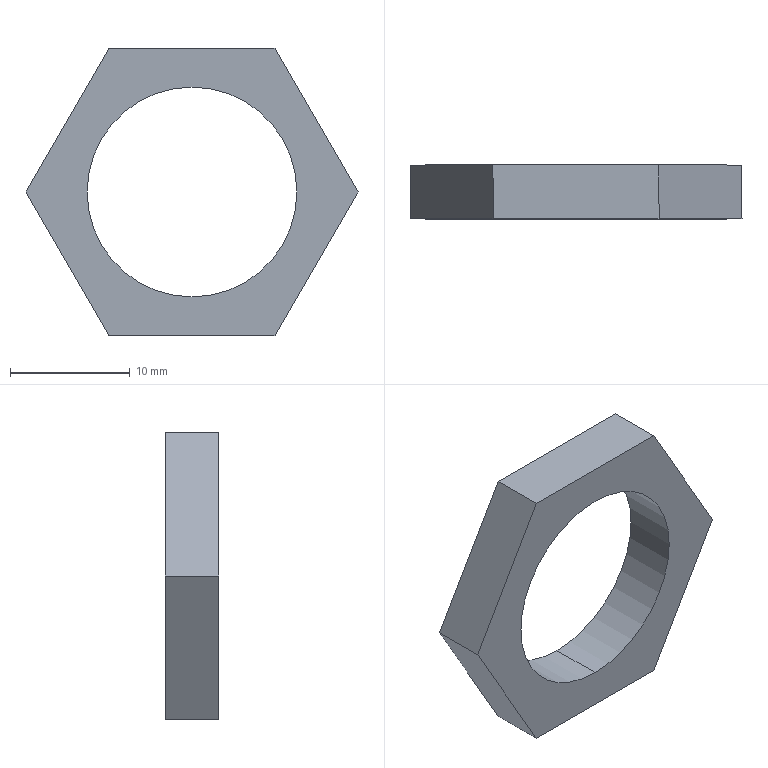Part | STEP file | Screen clamp lock nut 002 | 1 solid | 10 faces | box 27.713 x 4.5 x 24 mm | volume 1162 mm3 | plane 8 | cylinder 2 | commonest cylinder face diameters 17.5 x2
STEP:
#1=CARTESIAN_POINT('',(-319.123,-1225.634,-13247.04));
#2=VERTEX_POINT('',#1);
#3=CARTESIAN_POINT('',(-319.123,-1225.634,-13229.54));
#4=VERTEX_POINT('',#3);
#5=CARTESIAN_POINT('',(-319.123,-1225.634,-13238.29));
#6=DIRECTION('',(0.,1.,0.));
#7=DIRECTION('',(-1.,0.,0.));
#8=AXIS2_PLACEMENT_3D('',#5,#6,#7);
#9=CIRCLE('',#8,8.75);
#10=EDGE_CURVE('',#2,#4,#9,.T.);
#11=ORIENTED_EDGE('',*,*,#10,.F.);
#12=CARTESIAN_POINT('',(-319.123,-1221.134,-13247.04));
#13=VERTEX_POINT('',#12);
#14=CARTESIAN_POINT('',(-319.123,-1221.134,-13247.04));
#15=DIRECTION('',(0.,1.,0.));
#16=VECTOR('',#15,1000.);
#17=LINE('',#14,#16);
#18=EDGE_CURVE('',#2,#13,#17,.T.);
#19=ORIENTED_EDGE('',*,*,#18,.T.);
#20=CARTESIAN_POINT('',(-319.123,-1221.134,-13229.54));
#21=VERTEX_POINT('',#20);
#22=CARTESIAN_POINT('',(-319.123,-1221.134,-13238.29));
#23=DIRECTION('',(0.,1.,0.));
#24=DIRECTION('',(0.,0.,1.));
#25=AXIS2_PLACEMENT_3D('',#22,#23,#24);
#26=CIRCLE('',#25,8.75);
#27=EDGE_CURVE('',#13,#21,#26,.T.);
#28=ORIENTED_EDGE('',*,*,#27,.T.);
#29=CARTESIAN_POINT('',(-319.123,-1221.134,-13229.54));
#30=DIRECTION('',(0.,1.,0.));
#31=VECTOR('',#30,1000.);
#32=LINE('',#29,#31);
#33=EDGE_CURVE('',#4,#21,#32,.T.);
#34=ORIENTED_EDGE('',*,*,#33,.F.);
#35=EDGE_LOOP('',(#11,#19,#28,#34));
#36=FACE_OUTER_BOUND('',#35,.T.);
#37=CARTESIAN_POINT('',(-319.123,-1221.134,-13238.29));
#38=DIRECTION('',(0.,1.,0.));
#39=DIRECTION('',(0.,0.,1.));
#40=AXIS2_PLACEMENT_3D('',#37,#38,#39);
#41=CYLINDRICAL_SURFACE('',#40,8.75);
#42=ADVANCED_FACE('',(#36),#41,.F.);
#43=CARTESIAN_POINT('',(-326.051,-1225.634,-13250.29));
#44=VERTEX_POINT('',#43);
#45=CARTESIAN_POINT('',(-332.979,-1225.634,-13238.29));
#46=VERTEX_POINT('',#45);
#47=CARTESIAN_POINT('',(-326.051,-1225.634,-13250.29));
#48=DIRECTION('',(-0.5,0.,0.866));
#49=VECTOR('',#48,1000.);
#50=LINE('',#47,#49);
#51=EDGE_CURVE('',#44,#46,#50,.T.);
#52=ORIENTED_EDGE('',*,*,#51,.T.);
#53=CARTESIAN_POINT('',(-332.979,-1221.134,-13238.29));
#54=VERTEX_POINT('',#53);
#55=CARTESIAN_POINT('',(-332.979,-1221.134,-13238.29));
#56=DIRECTION('',(0.,-1.,0.));
#57=VECTOR('',#56,1000.);
#58=LINE('',#55,#57);
#59=EDGE_CURVE('',#54,#46,#58,.T.);
#60=ORIENTED_EDGE('',*,*,#59,.F.);
#61=CARTESIAN_POINT('',(-326.051,-1221.134,-13250.29));
#62=VERTEX_POINT('',#61);
#63=CARTESIAN_POINT('',(-326.051,-1221.134,-13250.29));
#64=DIRECTION('',(-0.5,0.,0.866));
#65=VECTOR('',#64,1000.);
#66=LINE('',#63,#65);
#67=EDGE_CURVE('',#62,#54,#66,.T.);
#68=ORIENTED_EDGE('',*,*,#67,.F.);
#69=CARTESIAN_POINT('',(-326.051,-1221.134,-13250.29));
#70=DIRECTION('',(0.,-1.,0.));
#71=VECTOR('',#70,1000.);
#72=LINE('',#69,#71);
#73=EDGE_CURVE('',#62,#44,#72,.T.);
#74=ORIENTED_EDGE('',*,*,#73,.T.);
#75=EDGE_LOOP('',(#52,#60,#68,#74));
#76=FACE_OUTER_BOUND('',#75,.T.);
#77=CARTESIAN_POINT('',(-326.051,-1221.134,-13250.29));
#78=DIRECTION('',(0.866,0.,0.5));
#79=DIRECTION('',(0.5,0.,-0.866));
#80=AXIS2_PLACEMENT_3D('',#77,#78,#79);
#81=PLANE('',#80);
#82=ADVANCED_FACE('',(#76),#81,.F.);
#83=CARTESIAN_POINT('',(-326.051,-1225.634,-13226.29));
#84=VERTEX_POINT('',#83);
#85=CARTESIAN_POINT('',(-332.979,-1225.634,-13238.29));
#86=DIRECTION('',(0.5,0.,0.866));
#87=VECTOR('',#86,1000.);
#88=LINE('',#85,#87);
#89=EDGE_CURVE('',#46,#84,#88,.T.);
#90=ORIENTED_EDGE('',*,*,#89,.T.);
#91=CARTESIAN_POINT('',(-326.051,-1221.134,-13226.29));
#92=VERTEX_POINT('',#91);
#93=CARTESIAN_POINT('',(-326.051,-1221.134,-13226.29));
#94=DIRECTION('',(0.,-1.,0.));
#95=VECTOR('',#94,1000.);
#96=LINE('',#93,#95);
#97=EDGE_CURVE('',#92,#84,#96,.T.);
#98=ORIENTED_EDGE('',*,*,#97,.F.);
#99=CARTESIAN_POINT('',(-332.979,-1221.134,-13238.29));
#100=DIRECTION('',(0.5,0.,0.866));
#101=VECTOR('',#100,1000.);
#102=LINE('',#99,#101);
#103=EDGE_CURVE('',#54,#92,#102,.T.);
#104=ORIENTED_EDGE('',*,*,#103,.F.);
#105=ORIENTED_EDGE('',*,*,#59,.T.);
#106=EDGE_LOOP('',(#90,#98,#104,#105));
#107=FACE_OUTER_BOUND('',#106,.T.);
#108=CARTESIAN_POINT('',(-332.979,-1221.134,-13238.29));
#109=DIRECTION('',(0.866,0.,-0.5));
#110=DIRECTION('',(-0.5,0.,-0.866));
#111=AXIS2_PLACEMENT_3D('',#108,#109,#110);
#112=PLANE('',#111);
#113=ADVANCED_FACE('',(#107),#112,.F.);
#114=CARTESIAN_POINT('',(-312.194,-1225.634,-13226.29));
#115=VERTEX_POINT('',#114);
#116=CARTESIAN_POINT('',(-326.051,-1225.634,-13226.29));
#117=DIRECTION('',(1.,0.,0.));
#118=VECTOR('',#117,1000.);
#119=LINE('',#116,#118);
#120=EDGE_CURVE('',#84,#115,#119,.T.);
#121=ORIENTED_EDGE('',*,*,#120,.T.);
#122=CARTESIAN_POINT('',(-312.194,-1221.134,-13226.29));
#123=VERTEX_POINT('',#122);
#124=CARTESIAN_POINT('',(-312.194,-1221.134,-13226.29));
#125=DIRECTION('',(0.,-1.,0.));
#126=VECTOR('',#125,1000.);
#127=LINE('',#124,#126);
#128=EDGE_CURVE('',#123,#115,#127,.T.);
#129=ORIENTED_EDGE('',*,*,#128,.F.);
#130=CARTESIAN_POINT('',(-326.051,-1221.134,-13226.29));
#131=DIRECTION('',(1.,0.,0.));
#132=VECTOR('',#131,1000.);
#133=LINE('',#130,#132);
#134=EDGE_CURVE('',#92,#123,#133,.T.);
#135=ORIENTED_EDGE('',*,*,#134,.F.);
#136=ORIENTED_EDGE('',*,*,#97,.T.);
#137=EDGE_LOOP('',(#121,#129,#135,#136));
#138=FACE_OUTER_BOUND('',#137,.T.);
#139=CARTESIAN_POINT('',(-326.051,-1221.134,-13226.29));
#140=DIRECTION('',(0.,0.,-1.));
#141=DIRECTION('',(0.,1.,0.));
#142=AXIS2_PLACEMENT_3D('',#139,#140,#141);
#143=PLANE('',#142);
#144=ADVANCED_FACE('',(#138),#143,.F.);
#145=CARTESIAN_POINT('',(-305.266,-1225.634,-13238.29));
#146=VERTEX_POINT('',#145);
#147=CARTESIAN_POINT('',(-312.194,-1225.634,-13226.29));
#148=DIRECTION('',(0.5,0.,-0.866));
#149=VECTOR('',#148,1000.);
#150=LINE('',#147,#149);
#151=EDGE_CURVE('',#115,#146,#150,.T.);
#152=ORIENTED_EDGE('',*,*,#151,.T.);
#153=CARTESIAN_POINT('',(-305.266,-1221.134,-13238.29));
#154=VERTEX_POINT('',#153);
#155=CARTESIAN_POINT('',(-305.266,-1221.134,-13238.29));
#156=DIRECTION('',(0.,-1.,0.));
#157=VECTOR('',#156,1000.);
#158=LINE('',#155,#157);
#159=EDGE_CURVE('',#154,#146,#158,.T.);
#160=ORIENTED_EDGE('',*,*,#159,.F.);
#161=CARTESIAN_POINT('',(-312.194,-1221.134,-13226.29));
#162=DIRECTION('',(0.5,0.,-0.866));
#163=VECTOR('',#162,1000.);
#164=LINE('',#161,#163);
#165=EDGE_CURVE('',#123,#154,#164,.T.);
#166=ORIENTED_EDGE('',*,*,#165,.F.);
#167=ORIENTED_EDGE('',*,*,#128,.T.);
#168=EDGE_LOOP('',(#152,#160,#166,#167));
#169=FACE_OUTER_BOUND('',#168,.T.);
#170=CARTESIAN_POINT('',(-312.194,-1221.134,-13226.29));
#171=DIRECTION('',(-0.866,0.,-0.5));
#172=DIRECTION('',(-0.5,0.,0.866));
#173=AXIS2_PLACEMENT_3D('',#170,#171,#172);
#174=PLANE('',#173);
#175=ADVANCED_FACE('',(#169),#174,.F.);
#176=CARTESIAN_POINT('',(-312.194,-1225.634,-13250.29));
#177=VERTEX_POINT('',#176);
#178=CARTESIAN_POINT('',(-305.266,-1225.634,-13238.29));
#179=DIRECTION('',(-0.5,0.,-0.866));
#180=VECTOR('',#179,1000.);
#181=LINE('',#178,#180);
#182=EDGE_CURVE('',#146,#177,#181,.T.);
#183=ORIENTED_EDGE('',*,*,#182,.T.);
#184=CARTESIAN_POINT('',(-312.194,-1221.134,-13250.29));
#185=VERTEX_POINT('',#184);
#186=CARTESIAN_POINT('',(-312.194,-1221.134,-13250.29));
#187=DIRECTION('',(0.,-1.,0.));
#188=VECTOR('',#187,1000.);
#189=LINE('',#186,#188);
#190=EDGE_CURVE('',#185,#177,#189,.T.);
#191=ORIENTED_EDGE('',*,*,#190,.F.);
#192=CARTESIAN_POINT('',(-305.266,-1221.134,-13238.29));
#193=DIRECTION('',(-0.5,0.,-0.866));
#194=VECTOR('',#193,1000.);
#195=LINE('',#192,#194);
#196=EDGE_CURVE('',#154,#185,#195,.T.);
#197=ORIENTED_EDGE('',*,*,#196,.F.);
#198=ORIENTED_EDGE('',*,*,#159,.T.);
#199=EDGE_LOOP('',(#183,#191,#197,#198));
#200=FACE_OUTER_BOUND('',#199,.T.);
#201=CARTESIAN_POINT('',(-305.266,-1221.134,-13238.29));
#202=DIRECTION('',(-0.866,0.,0.5));
#203=DIRECTION('',(0.5,0.,0.866));
#204=AXIS2_PLACEMENT_3D('',#201,#202,#203);
#205=PLANE('',#204);
#206=ADVANCED_FACE('',(#200),#205,.F.);
#207=CARTESIAN_POINT('',(-312.194,-1225.634,-13250.29));
#208=DIRECTION('',(-1.,0.,0.));
#209=VECTOR('',#208,1000.);
#210=LINE('',#207,#209);
#211=EDGE_CURVE('',#177,#44,#210,.T.);
#212=ORIENTED_EDGE('',*,*,#211,.T.);
#213=ORIENTED_EDGE('',*,*,#73,.F.);
#214=CARTESIAN_POINT('',(-312.194,-1221.134,-13250.29));
#215=DIRECTION('',(-1.,0.,0.));
#216=VECTOR('',#215,1000.);
#217=LINE('',#214,#216);
#218=EDGE_CURVE('',#185,#62,#217,.T.);
#219=ORIENTED_EDGE('',*,*,#218,.F.);
#220=ORIENTED_EDGE('',*,*,#190,.T.);
#221=EDGE_LOOP('',(#212,#213,#219,#220));
#222=FACE_OUTER_BOUND('',#221,.T.);
#223=CARTESIAN_POINT('',(-312.194,-1221.134,-13250.29));
#224=DIRECTION('',(0.,0.,1.));
#225=DIRECTION('',(1.,0.,0.));
#226=AXIS2_PLACEMENT_3D('',#223,#224,#225);
#227=PLANE('',#226);
#228=ADVANCED_FACE('',(#222),#227,.F.);
#229=CARTESIAN_POINT('',(-319.123,-1221.134,-13238.29));
#230=DIRECTION('',(0.,1.,0.));
#231=DIRECTION('',(0.,0.,1.));
#232=AXIS2_PLACEMENT_3D('',#229,#230,#231);
#233=CIRCLE('',#232,8.75);
#234=EDGE_CURVE('',#21,#13,#233,.T.);
#235=ORIENTED_EDGE('',*,*,#234,.F.);
#236=ORIENTED_EDGE('',*,*,#27,.F.);
#237=EDGE_LOOP('',(#235,#236));
#238=FACE_BOUND('',#237,.T.);
#239=ORIENTED_EDGE('',*,*,#67,.T.);
#240=ORIENTED_EDGE('',*,*,#103,.T.);
#241=ORIENTED_EDGE('',*,*,#134,.T.);
#242=ORIENTED_EDGE('',*,*,#165,.T.);
#243=ORIENTED_EDGE('',*,*,#196,.T.);
#244=ORIENTED_EDGE('',*,*,#218,.T.);
#245=EDGE_LOOP('',(#239,#240,#241,#242,#243,#244));
#246=FACE_OUTER_BOUND('',#245,.T.);
#247=CARTESIAN_POINT('',(-332.979,-1221.134,-13238.29));
#248=DIRECTION('',(0.,1.,0.));
#249=DIRECTION('',(-1.,0.,0.));
#250=AXIS2_PLACEMENT_3D('',#247,#248,#249);
#251=PLANE('',#250);
#252=ADVANCED_FACE('',(#238,#246),#251,.T.);
#253=CARTESIAN_POINT('',(-319.123,-1225.634,-13238.29));
#254=DIRECTION('',(0.,1.,0.));
#255=DIRECTION('',(-1.,0.,0.));
#256=AXIS2_PLACEMENT_3D('',#253,#254,#255);
#257=CIRCLE('',#256,8.75);
#258=EDGE_CURVE('',#4,#2,#257,.T.);
#259=ORIENTED_EDGE('',*,*,#258,.T.);
#260=ORIENTED_EDGE('',*,*,#10,.T.);
#261=EDGE_LOOP('',(#259,#260));
#262=FACE_BOUND('',#261,.T.);
#263=ORIENTED_EDGE('',*,*,#51,.F.);
#264=ORIENTED_EDGE('',*,*,#211,.F.);
#265=ORIENTED_EDGE('',*,*,#182,.F.);
#266=ORIENTED_EDGE('',*,*,#151,.F.);
#267=ORIENTED_EDGE('',*,*,#120,.F.);
#268=ORIENTED_EDGE('',*,*,#89,.F.);
#269=EDGE_LOOP('',(#263,#264,#265,#266,#267,#268));
#270=FACE_OUTER_BOUND('',#269,.T.);
#271=CARTESIAN_POINT('',(-332.979,-1225.634,-13238.29));
#272=DIRECTION('',(0.,1.,0.));
#273=DIRECTION('',(-1.,0.,0.));
#274=AXIS2_PLACEMENT_3D('',#271,#272,#273);
#275=PLANE('',#274);
#276=ADVANCED_FACE('',(#262,#270),#275,.F.);
#277=ORIENTED_EDGE('',*,*,#18,.F.);
#278=ORIENTED_EDGE('',*,*,#258,.F.);
#279=ORIENTED_EDGE('',*,*,#33,.T.);
#280=ORIENTED_EDGE('',*,*,#234,.T.);
#281=EDGE_LOOP('',(#277,#278,#279,#280));
#282=FACE_OUTER_BOUND('',#281,.T.);
#283=CARTESIAN_POINT('',(-319.123,-1221.134,-13238.29));
#284=DIRECTION('',(0.,1.,0.));
#285=DIRECTION('',(0.,0.,1.));
#286=AXIS2_PLACEMENT_3D('',#283,#284,#285);
#287=CYLINDRICAL_SURFACE('',#286,8.75);
#288=ADVANCED_FACE('',(#282),#287,.F.);
#289=CLOSED_SHELL('',(#42,#82,#113,#144,#175,#206,#228,#252,#276,#288));
#290=MANIFOLD_SOLID_BREP('',#289);
#291=CARTESIAN_POINT('',(0.,0.,0.));
#292=DIRECTION('',(0.,0.,1.));
#293=DIRECTION('',(1.,0.,0.));
#294=AXIS2_PLACEMENT_3D('',#291,#292,#293);
#295=(LENGTH_UNIT()NAMED_UNIT(*)SI_UNIT(.MILLI.,.METRE.));
#296=UNCERTAINTY_MEASURE_WITH_UNIT(LENGTH_MEASURE(0.00001),#295,'','');
#297=(NAMED_UNIT(*)PLANE_ANGLE_UNIT()SI_UNIT($,.RADIAN.));
#298=(NAMED_UNIT(*)SI_UNIT($,.STERADIAN.)SOLID_ANGLE_UNIT());
#299=(GEOMETRIC_REPRESENTATION_CONTEXT(3)GLOBAL_UNCERTAINTY_ASSIGNED_CONTEXT((#296))GLOBAL_UNIT_ASSIGNED_CONTEXT((#295,#297,#298))REPRESENTATION_CONTEXT('',''));
#300=ADVANCED_BREP_SHAPE_REPRESENTATION('',(#290,#294),#299);